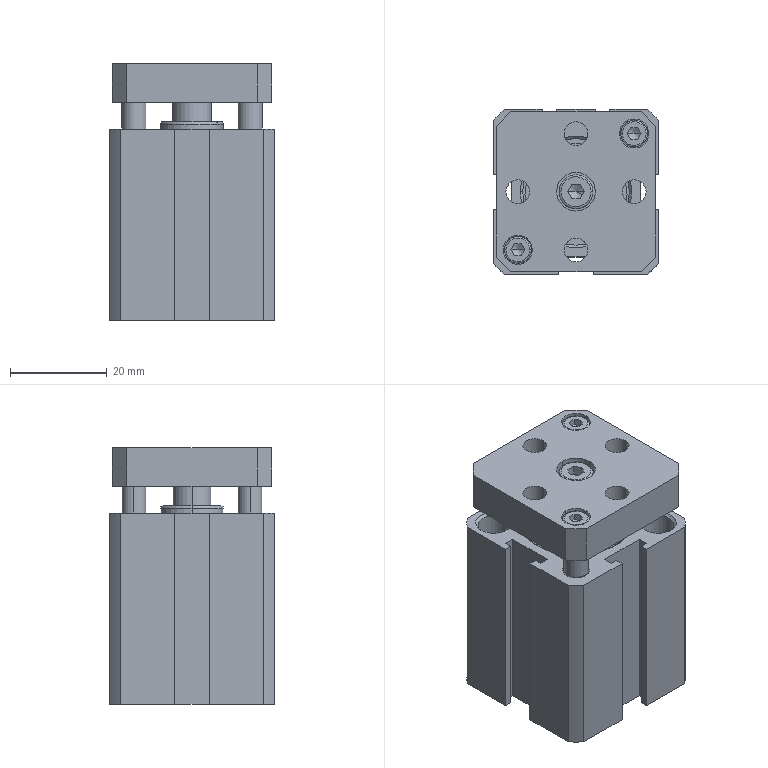Part | SolidWorks | 6 solids | 262 faces | box 34 x 34 x 53 mm | volume 43812 mm3 | cylinder 116 | plane 104 | cone 28 | spline 10 | torus 4 | commonest cylinder face diameters 3 x14 1.5 x12 4.917 x8 5.5 x8 6.5 x8 22 x8